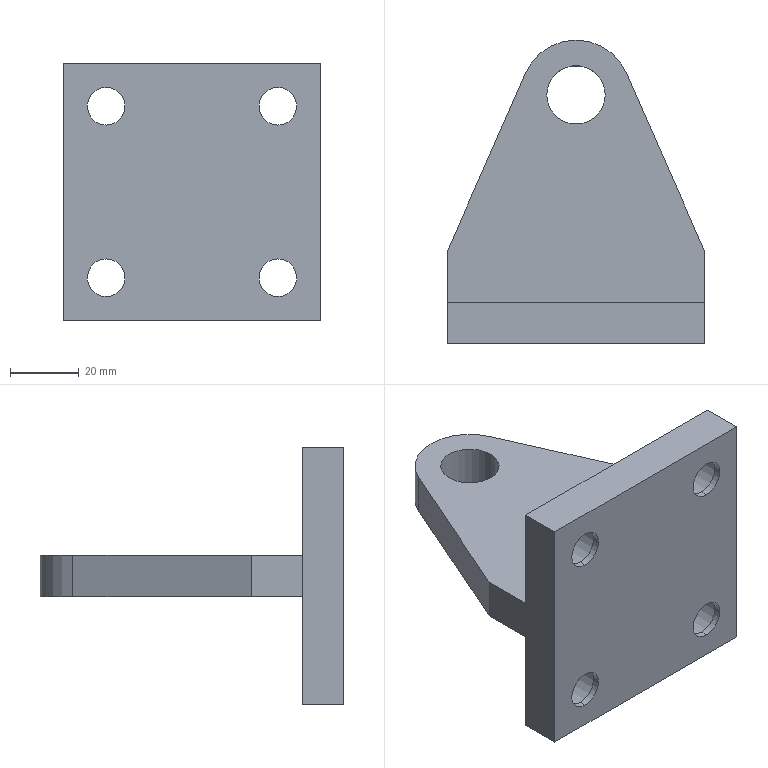Part | SolidWorks | features ICE 3, Extrusion 1, HoleWzd 1 | 2 solids | 36 faces | box 75 x 88.5 x 75 mm | volume 103360 mm3 | cylinder 19 | plane 17 | commonest cylinder face diameters 17 x10 11 x8 32 x1
STEP:
#1=CARTESIAN_POINT('',(-8.5,72.5,-6.));
#2=VERTEX_POINT('',#1);
#3=CARTESIAN_POINT('',(8.5,72.5,-6.));
#4=VERTEX_POINT('',#3);
#5=CARTESIAN_POINT('',(0.,72.5,-6.));
#6=DIRECTION('',(0.,0.,1.));
#7=DIRECTION('',(1.,0.,0.));
#8=AXIS2_PLACEMENT_3D('',#5,#6,#7);
#9=CIRCLE('',#8,8.5);
#10=EDGE_CURVE('',#2,#4,#9,.T.);
#11=ORIENTED_EDGE('',*,*,#10,.F.);
#12=CARTESIAN_POINT('',(-8.5,72.5,6.));
#13=VERTEX_POINT('',#12);
#14=CARTESIAN_POINT('',(-8.5,72.5,-37.5));
#15=DIRECTION('',(0.,0.,1.));
#16=VECTOR('',#15,1000.);
#17=LINE('',#14,#16);
#18=EDGE_CURVE('',#2,#13,#17,.T.);
#19=ORIENTED_EDGE('',*,*,#18,.T.);
#20=CARTESIAN_POINT('',(8.5,72.5,6.));
#21=VERTEX_POINT('',#20);
#22=CARTESIAN_POINT('',(0.,72.5,6.));
#23=DIRECTION('',(0.,0.,1.));
#24=DIRECTION('',(1.,0.,0.));
#25=AXIS2_PLACEMENT_3D('',#22,#23,#24);
#26=CIRCLE('',#25,8.5);
#27=EDGE_CURVE('',#13,#21,#26,.T.);
#28=ORIENTED_EDGE('',*,*,#27,.T.);
#29=CARTESIAN_POINT('',(8.5,72.5,-37.5));
#30=DIRECTION('',(0.,0.,1.));
#31=VECTOR('',#30,1000.);
#32=LINE('',#29,#31);
#33=EDGE_CURVE('',#4,#21,#32,.T.);
#34=ORIENTED_EDGE('',*,*,#33,.F.);
#35=EDGE_LOOP('',(#11,#19,#28,#34));
#36=FACE_OUTER_BOUND('',#35,.T.);
#37=CARTESIAN_POINT('',(0.,72.5,-37.5));
#38=DIRECTION('',(0.,0.,1.));
#39=DIRECTION('',(1.,0.,0.));
#40=AXIS2_PLACEMENT_3D('',#37,#38,#39);
#41=CYLINDRICAL_SURFACE('',#40,8.5);
#42=ADVANCED_FACE('',(#36),#41,.F.);
#43=CARTESIAN_POINT('',(37.5,27.,-6.));
#44=VERTEX_POINT('',#43);
#45=CARTESIAN_POINT('',(37.5,12.,-6.));
#46=VERTEX_POINT('',#45);
#47=CARTESIAN_POINT('',(37.5,88.5,-6.));
#48=DIRECTION('',(0.,-1.,0.));
#49=VECTOR('',#48,1000.);
#50=LINE('',#47,#49);
#51=EDGE_CURVE('',#44,#46,#50,.T.);
#52=ORIENTED_EDGE('',*,*,#51,.F.);
#53=CARTESIAN_POINT('',(37.5,27.,6.));
#54=VERTEX_POINT('',#53);
#55=CARTESIAN_POINT('',(37.5,27.,-37.5));
#56=DIRECTION('',(0.,0.,1.));
#57=VECTOR('',#56,1000.);
#58=LINE('',#55,#57);
#59=EDGE_CURVE('',#44,#54,#58,.T.);
#60=ORIENTED_EDGE('',*,*,#59,.T.);
#61=CARTESIAN_POINT('',(37.5,12.,6.));
#62=VERTEX_POINT('',#61);
#63=CARTESIAN_POINT('',(37.5,88.5,6.));
#64=DIRECTION('',(0.,-1.,0.));
#65=VECTOR('',#64,1000.);
#66=LINE('',#63,#65);
#67=EDGE_CURVE('',#54,#62,#66,.T.);
#68=ORIENTED_EDGE('',*,*,#67,.T.);
#69=CARTESIAN_POINT('',(37.5,12.,-6.));
#70=DIRECTION('',(0.,0.,-1.));
#71=VECTOR('',#70,1000.);
#72=LINE('',#69,#71);
#73=EDGE_CURVE('',#62,#46,#72,.T.);
#74=ORIENTED_EDGE('',*,*,#73,.T.);
#75=EDGE_LOOP('',(#52,#60,#68,#74));
#76=FACE_OUTER_BOUND('',#75,.T.);
#77=CARTESIAN_POINT('',(37.5,88.5,-6.));
#78=DIRECTION('',(-1.,0.,0.));
#79=DIRECTION('',(0.,0.,1.));
#80=AXIS2_PLACEMENT_3D('',#77,#78,#79);
#81=PLANE('',#80);
#82=ADVANCED_FACE('',(#76),#81,.F.);
#83=CARTESIAN_POINT('',(0.,72.5,-6.));
#84=DIRECTION('',(0.,0.,1.));
#85=DIRECTION('',(1.,0.,0.));
#86=AXIS2_PLACEMENT_3D('',#83,#84,#85);
#87=CIRCLE('',#86,8.5);
#88=EDGE_CURVE('',#4,#2,#87,.T.);
#89=ORIENTED_EDGE('',*,*,#88,.T.);
#90=ORIENTED_EDGE('',*,*,#10,.T.);
#91=EDGE_LOOP('',(#89,#90));
#92=FACE_BOUND('',#91,.T.);
#93=CARTESIAN_POINT('',(-37.5,27.,-6.));
#94=VERTEX_POINT('',#93);
#95=CARTESIAN_POINT('',(-37.5,12.,-6.));
#96=VERTEX_POINT('',#95);
#97=CARTESIAN_POINT('',(-37.5,88.5,-6.));
#98=DIRECTION('',(0.,-1.,0.));
#99=VECTOR('',#98,1000.);
#100=LINE('',#97,#99);
#101=EDGE_CURVE('',#94,#96,#100,.T.);
#102=ORIENTED_EDGE('',*,*,#101,.F.);
#103=CARTESIAN_POINT('',(-14.645,78.944,-6.));
#104=VERTEX_POINT('',#103);
#105=CARTESIAN_POINT('',(-14.829,78.525,-6.));
#106=DIRECTION('',(0.4027,0.9153,0.));
#107=VECTOR('',#106,1000.);
#108=LINE('',#105,#107);
#109=EDGE_CURVE('',#94,#104,#108,.T.);
#110=ORIENTED_EDGE('',*,*,#109,.T.);
#111=CARTESIAN_POINT('',(14.645,78.944,-6.));
#112=VERTEX_POINT('',#111);
#113=CARTESIAN_POINT('',(0.,72.5,-6.));
#114=DIRECTION('',(0.,0.,-1.));
#115=DIRECTION('',(1.,0.,0.));
#116=AXIS2_PLACEMENT_3D('',#113,#114,#115);
#117=CIRCLE('',#116,16.);
#118=EDGE_CURVE('',#104,#112,#117,.T.);
#119=ORIENTED_EDGE('',*,*,#118,.T.);
#120=CARTESIAN_POINT('',(2.665,106.172,-6.));
#121=DIRECTION('',(0.4027,-0.9153,0.));
#122=VECTOR('',#121,1000.);
#123=LINE('',#120,#122);
#124=EDGE_CURVE('',#112,#44,#123,.T.);
#125=ORIENTED_EDGE('',*,*,#124,.T.);
#126=ORIENTED_EDGE('',*,*,#51,.T.);
#127=CARTESIAN_POINT('',(-37.5,12.,-6.));
#128=DIRECTION('',(-1.,0.,0.));
#129=VECTOR('',#128,1000.);
#130=LINE('',#127,#129);
#131=EDGE_CURVE('',#46,#96,#130,.T.);
#132=ORIENTED_EDGE('',*,*,#131,.T.);
#133=EDGE_LOOP('',(#102,#110,#119,#125,#126,#132));
#134=FACE_OUTER_BOUND('',#133,.T.);
#135=CARTESIAN_POINT('',(-37.5,88.5,-6.));
#136=DIRECTION('',(0.,0.,1.));
#137=DIRECTION('',(1.,0.,0.));
#138=AXIS2_PLACEMENT_3D('',#135,#136,#137);
#139=PLANE('',#138);
#140=ADVANCED_FACE('',(#92,#134),#139,.F.);
#141=CARTESIAN_POINT('',(-37.5,27.,6.));
#142=VERTEX_POINT('',#141);
#143=CARTESIAN_POINT('',(-37.5,12.,6.));
#144=VERTEX_POINT('',#143);
#145=CARTESIAN_POINT('',(-37.5,88.5,6.));
#146=DIRECTION('',(0.,-1.,0.));
#147=VECTOR('',#146,1000.);
#148=LINE('',#145,#147);
#149=EDGE_CURVE('',#142,#144,#148,.T.);
#150=ORIENTED_EDGE('',*,*,#149,.F.);
#151=CARTESIAN_POINT('',(-37.5,27.,-37.5));
#152=DIRECTION('',(0.,0.,1.));
#153=VECTOR('',#152,1000.);
#154=LINE('',#151,#153);
#155=EDGE_CURVE('',#94,#142,#154,.T.);
#156=ORIENTED_EDGE('',*,*,#155,.F.);
#157=ORIENTED_EDGE('',*,*,#101,.T.);
#158=CARTESIAN_POINT('',(-37.5,12.,-6.));
#159=DIRECTION('',(0.,0.,1.));
#160=VECTOR('',#159,1000.);
#161=LINE('',#158,#160);
#162=EDGE_CURVE('',#96,#144,#161,.T.);
#163=ORIENTED_EDGE('',*,*,#162,.T.);
#164=EDGE_LOOP('',(#150,#156,#157,#163));
#165=FACE_OUTER_BOUND('',#164,.T.);
#166=CARTESIAN_POINT('',(-37.5,88.5,-6.));
#167=DIRECTION('',(1.,0.,0.));
#168=DIRECTION('',(0.,0.,-1.));
#169=AXIS2_PLACEMENT_3D('',#166,#167,#168);
#170=PLANE('',#169);
#171=ADVANCED_FACE('',(#165),#170,.F.);
#172=CARTESIAN_POINT('',(0.,72.5,6.));
#173=DIRECTION('',(0.,0.,1.));
#174=DIRECTION('',(1.,0.,0.));
#175=AXIS2_PLACEMENT_3D('',#172,#173,#174);
#176=CIRCLE('',#175,8.5);
#177=EDGE_CURVE('',#21,#13,#176,.T.);
#178=ORIENTED_EDGE('',*,*,#177,.F.);
#179=ORIENTED_EDGE('',*,*,#27,.F.);
#180=EDGE_LOOP('',(#178,#179));
#181=FACE_BOUND('',#180,.T.);
#182=CARTESIAN_POINT('',(-14.645,78.944,6.));
#183=VERTEX_POINT('',#182);
#184=CARTESIAN_POINT('',(14.645,78.944,6.));
#185=VERTEX_POINT('',#184);
#186=CARTESIAN_POINT('',(0.,72.5,6.));
#187=DIRECTION('',(0.,0.,-1.));
#188=DIRECTION('',(1.,0.,0.));
#189=AXIS2_PLACEMENT_3D('',#186,#187,#188);
#190=CIRCLE('',#189,16.);
#191=EDGE_CURVE('',#183,#185,#190,.T.);
#192=ORIENTED_EDGE('',*,*,#191,.F.);
#193=CARTESIAN_POINT('',(-37.5,27.,6.));
#194=DIRECTION('',(0.4027,0.9153,0.));
#195=VECTOR('',#194,1000.);
#196=LINE('',#193,#195);
#197=EDGE_CURVE('',#142,#183,#196,.T.);
#198=ORIENTED_EDGE('',*,*,#197,.F.);
#199=ORIENTED_EDGE('',*,*,#149,.T.);
#200=CARTESIAN_POINT('',(-37.5,12.,6.));
#201=DIRECTION('',(1.,0.,0.));
#202=VECTOR('',#201,1000.);
#203=LINE('',#200,#202);
#204=EDGE_CURVE('',#144,#62,#203,.T.);
#205=ORIENTED_EDGE('',*,*,#204,.T.);
#206=ORIENTED_EDGE('',*,*,#67,.F.);
#207=CARTESIAN_POINT('',(37.5,27.,6.));
#208=DIRECTION('',(0.4027,-0.9153,0.));
#209=VECTOR('',#208,1000.);
#210=LINE('',#207,#209);
#211=EDGE_CURVE('',#185,#54,#210,.T.);
#212=ORIENTED_EDGE('',*,*,#211,.F.);
#213=EDGE_LOOP('',(#192,#198,#199,#205,#206,#212));
#214=FACE_OUTER_BOUND('',#213,.T.);
#215=CARTESIAN_POINT('',(-37.5,88.5,6.));
#216=DIRECTION('',(0.,0.,-1.));
#217=DIRECTION('',(-1.,0.,0.));
#218=AXIS2_PLACEMENT_3D('',#215,#216,#217);
#219=PLANE('',#218);
#220=ADVANCED_FACE('',(#181,#214),#219,.F.);
#221=ORIENTED_EDGE('',*,*,#73,.F.);
#222=ORIENTED_EDGE('',*,*,#204,.F.);
#223=ORIENTED_EDGE('',*,*,#162,.F.);
#224=ORIENTED_EDGE('',*,*,#131,.F.);
#225=EDGE_LOOP('',(#221,#222,#223,#224));
#226=FACE_OUTER_BOUND('',#225,.T.);
#227=CARTESIAN_POINT('',(0.,12.,0.));
#228=DIRECTION('',(0.,1.,0.));
#229=DIRECTION('',(0.,0.,1.));
#230=AXIS2_PLACEMENT_3D('',#227,#228,#229);
#231=PLANE('',#230);
#232=ADVANCED_FACE('',(#226),#231,.F.);
#233=ORIENTED_EDGE('',*,*,#18,.F.);
#234=ORIENTED_EDGE('',*,*,#88,.F.);
#235=ORIENTED_EDGE('',*,*,#33,.T.);
#236=ORIENTED_EDGE('',*,*,#177,.T.);
#237=EDGE_LOOP('',(#233,#234,#235,#236));
#238=FACE_OUTER_BOUND('',#237,.T.);
#239=CARTESIAN_POINT('',(0.,72.5,-37.5));
#240=DIRECTION('',(0.,0.,1.));
#241=DIRECTION('',(1.,0.,0.));
#242=AXIS2_PLACEMENT_3D('',#239,#240,#241);
#243=CYLINDRICAL_SURFACE('',#242,8.5);
#244=ADVANCED_FACE('',(#238),#243,.F.);
#245=ORIENTED_EDGE('',*,*,#155,.T.);
#246=ORIENTED_EDGE('',*,*,#197,.T.);
#247=CARTESIAN_POINT('',(-14.645,78.944,-37.5));
#248=DIRECTION('',(0.,0.,1.));
#249=VECTOR('',#248,1000.);
#250=LINE('',#247,#249);
#251=EDGE_CURVE('',#104,#183,#250,.T.);
#252=ORIENTED_EDGE('',*,*,#251,.F.);
#253=ORIENTED_EDGE('',*,*,#109,.F.);
#254=EDGE_LOOP('',(#245,#246,#252,#253));
#255=FACE_OUTER_BOUND('',#254,.T.);
#256=CARTESIAN_POINT('',(-37.5,27.,-37.5));
#257=DIRECTION('',(0.9153,-0.4027,0.));
#258=DIRECTION('',(0.4027,0.9153,0.));
#259=AXIS2_PLACEMENT_3D('',#256,#257,#258);
#260=PLANE('',#259);
#261=ADVANCED_FACE('',(#255),#260,.F.);
#262=CARTESIAN_POINT('',(14.645,78.944,-37.5));
#263=DIRECTION('',(0.,0.,1.));
#264=VECTOR('',#263,1000.);
#265=LINE('',#262,#264);
#266=EDGE_CURVE('',#112,#185,#265,.T.);
#267=ORIENTED_EDGE('',*,*,#266,.T.);
#268=ORIENTED_EDGE('',*,*,#211,.T.);
#269=ORIENTED_EDGE('',*,*,#59,.F.);
#270=ORIENTED_EDGE('',*,*,#124,.F.);
#271=EDGE_LOOP('',(#267,#268,#269,#270));
#272=FACE_OUTER_BOUND('',#271,.T.);
#273=CARTESIAN_POINT('',(37.5,27.,-37.5));
#274=DIRECTION('',(-0.9153,-0.4027,0.));
#275=DIRECTION('',(0.4027,-0.9153,0.));
#276=AXIS2_PLACEMENT_3D('',#273,#274,#275);
#277=PLANE('',#276);
#278=ADVANCED_FACE('',(#272),#277,.F.);
#279=ORIENTED_EDGE('',*,*,#251,.T.);
#280=ORIENTED_EDGE('',*,*,#191,.T.);
#281=ORIENTED_EDGE('',*,*,#266,.F.);
#282=ORIENTED_EDGE('',*,*,#118,.F.);
#283=EDGE_LOOP('',(#279,#280,#281,#282));
#284=FACE_OUTER_BOUND('',#283,.T.);
#285=CARTESIAN_POINT('',(0.,72.5,-37.5));
#286=DIRECTION('',(0.,0.,1.));
#287=DIRECTION('',(1.,0.,0.));
#288=AXIS2_PLACEMENT_3D('',#285,#286,#287);
#289=CYLINDRICAL_SURFACE('',#288,16.);
#290=ADVANCED_FACE('',(#284),#289,.T.);
#291=CLOSED_SHELL('',(#42,#82,#140,#171,#220,#232,#244,#261,#278,#290));
#292=MANIFOLD_SOLID_BREP('',#291);
#293=CARTESIAN_POINT('',(25.,2.,16.5));
#294=VERTEX_POINT('',#293);
#295=CARTESIAN_POINT('',(25.,2.,33.5));
#296=VERTEX_POINT('',#295);
#297=CARTESIAN_POINT('',(25.,2.,25.));
#298=DIRECTION('',(0.,1.,0.));
#299=DIRECTION('',(0.,0.,1.));
#300=AXIS2_PLACEMENT_3D('',#297,#298,#299);
#301=CIRCLE('',#300,8.5);
#302=EDGE_CURVE('',#294,#296,#301,.T.);
#303=ORIENTED_EDGE('',*,*,#302,.F.);
#304=CARTESIAN_POINT('',(25.,12.,16.5));
#305=VERTEX_POINT('',#304);
#306=CARTESIAN_POINT('',(25.,12.,16.5));
#307=DIRECTION('',(0.,1.,0.));
#308=VECTOR('',#307,1000.);
#309=LINE('',#306,#308);
#310=EDGE_CURVE('',#294,#305,#309,.T.);
#311=ORIENTED_EDGE('',*,*,#310,.T.);
#312=CARTESIAN_POINT('',(25.,12.,33.5));
#313=VERTEX_POINT('',#312);
#314=CARTESIAN_POINT('',(25.,12.,25.));
#315=DIRECTION('',(0.,1.,0.));
#316=DIRECTION('',(0.,0.,1.));
#317=AXIS2_PLACEMENT_3D('',#314,#315,#316);
#318=CIRCLE('',#317,8.5);
#319=EDGE_CURVE('',#305,#313,#318,.T.);
#320=ORIENTED_EDGE('',*,*,#319,.T.);
#321=CARTESIAN_POINT('',(25.,12.,33.5));
#322=DIRECTION('',(0.,1.,0.));
#323=VECTOR('',#322,1000.);
#324=LINE('',#321,#323);
#325=EDGE_CURVE('',#296,#313,#324,.T.);
#326=ORIENTED_EDGE('',*,*,#325,.F.);
#327=EDGE_LOOP('',(#303,#311,#320,#326));
#328=FACE_OUTER_BOUND('',#327,.T.);
#329=CARTESIAN_POINT('',(25.,12.,25.));
#330=DIRECTION('',(0.,1.,0.));
#331=DIRECTION('',(0.,0.,1.));
#332=AXIS2_PLACEMENT_3D('',#329,#330,#331);
#333=CYLINDRICAL_SURFACE('',#332,8.5);
#334=ADVANCED_FACE('',(#328),#333,.F.);
#335=CARTESIAN_POINT('',(25.,0.,19.5));
#336=VERTEX_POINT('',#335);
#337=CARTESIAN_POINT('',(25.,0.,30.5));
#338=VERTEX_POINT('',#337);
#339=CARTESIAN_POINT('',(25.,0.,25.));
#340=DIRECTION('',(0.,1.,0.));
#341=DIRECTION('',(0.,0.,1.));
#342=AXIS2_PLACEMENT_3D('',#339,#340,#341);
#343=CIRCLE('',#342,5.5);
#344=EDGE_CURVE('',#336,#338,#343,.T.);
#345=ORIENTED_EDGE('',*,*,#344,.F.);
#346=CARTESIAN_POINT('',(25.,2.,19.5));
#347=VERTEX_POINT('',#346);
#348=CARTESIAN_POINT('',(25.,12.,19.5));
#349=DIRECTION('',(0.,1.,0.));
#350=VECTOR('',#349,1000.);
#351=LINE('',#348,#350);
#352=EDGE_CURVE('',#336,#347,#351,.T.);
#353=ORIENTED_EDGE('',*,*,#352,.T.);
#354=CARTESIAN_POINT('',(25.,2.,30.5));
#355=VERTEX_POINT('',#354);
#356=CARTESIAN_POINT('',(25.,2.,25.));
#357=DIRECTION('',(0.,1.,0.));
#358=DIRECTION('',(0.,0.,1.));
#359=AXIS2_PLACEMENT_3D('',#356,#357,#358);
#360=CIRCLE('',#359,5.5);
#361=EDGE_CURVE('',#347,#355,#360,.T.);
#362=ORIENTED_EDGE('',*,*,#361,.T.);
#363=CARTESIAN_POINT('',(25.,12.,30.5));
#364=DIRECTION('',(0.,1.,0.));
#365=VECTOR('',#364,1000.);
#366=LINE('',#363,#365);
#367=EDGE_CURVE('',#338,#355,#366,.T.);
#368=ORIENTED_EDGE('',*,*,#367,.F.);
#369=EDGE_LOOP('',(#345,#353,#362,#368));
#370=FACE_OUTER_BOUND('',#369,.T.);
#371=CARTESIAN_POINT('',(25.,12.,25.));
#372=DIRECTION('',(0.,1.,0.));
#373=DIRECTION('',(0.,0.,1.));
#374=AXIS2_PLACEMENT_3D('',#371,#372,#373);
#375=CYLINDRICAL_SURFACE('',#374,5.5);
#376=ADVANCED_FACE('',(#370),#375,.F.);
#377=CARTESIAN_POINT('',(-25.,2.,-33.5));
#378=VERTEX_POINT('',#377);
#379=CARTESIAN_POINT('',(-25.,2.,-16.5));
#380=VERTEX_POINT('',#379);
#381=CARTESIAN_POINT('',(-25.,2.,-25.));
#382=DIRECTION('',(0.,1.,0.));
#383=DIRECTION('',(0.,0.,1.));
#384=AXIS2_PLACEMENT_3D('',#381,#382,#383);
#385=CIRCLE('',#384,8.5);
#386=EDGE_CURVE('',#378,#380,#385,.T.);
#387=ORIENTED_EDGE('',*,*,#386,.F.);
#388=CARTESIAN_POINT('',(-25.,12.,-33.5));
#389=VERTEX_POINT('',#388);
#390=CARTESIAN_POINT('',(-25.,12.,-33.5));
#391=DIRECTION('',(0.,1.,0.));
#392=VECTOR('',#391,1000.);
#393=LINE('',#390,#392);
#394=EDGE_CURVE('',#378,#389,#393,.T.);
#395=ORIENTED_EDGE('',*,*,#394,.T.);
#396=CARTESIAN_POINT('',(-25.,12.,-16.5));
#397=VERTEX_POINT('',#396);
#398=CARTESIAN_POINT('',(-25.,12.,-25.));
#399=DIRECTION('',(0.,1.,0.));
#400=DIRECTION('',(0.,0.,1.));
#401=AXIS2_PLACEMENT_3D('',#398,#399,#400);
#402=CIRCLE('',#401,8.5);
#403=EDGE_CURVE('',#389,#397,#402,.T.);
#404=ORIENTED_EDGE('',*,*,#403,.T.);
#405=CARTESIAN_POINT('',(-25.,12.,-16.5));
#406=DIRECTION('',(0.,1.,0.));
#407=VECTOR('',#406,1000.);
#408=LINE('',#405,#407);
#409=EDGE_CURVE('',#380,#397,#408,.T.);
#410=ORIENTED_EDGE('',*,*,#409,.F.);
#411=EDGE_LOOP('',(#387,#395,#404,#410));
#412=FACE_OUTER_BOUND('',#411,.T.);
#413=CARTESIAN_POINT('',(-25.,12.,-25.));
#414=DIRECTION('',(0.,1.,0.));
#415=DIRECTION('',(0.,0.,1.));
#416=AXIS2_PLACEMENT_3D('',#413,#414,#415);
#417=CYLINDRICAL_SURFACE('',#416,8.5);
#418=ADVANCED_FACE('',(#412),#417,.F.);
#419=CARTESIAN_POINT('',(-25.,0.,-30.5));
#420=VERTEX_POINT('',#419);
#421=CARTESIAN_POINT('',(-25.,0.,-19.5));
#422=VERTEX_POINT('',#421);
#423=CARTESIAN_POINT('',(-25.,0.,-25.));
#424=DIRECTION('',(0.,1.,0.));
#425=DIRECTION('',(0.,0.,1.));
#426=AXIS2_PLACEMENT_3D('',#423,#424,#425);
#427=CIRCLE('',#426,5.5);
#428=EDGE_CURVE('',#420,#422,#427,.T.);
#429=ORIENTED_EDGE('',*,*,#428,.F.);
#430=CARTESIAN_POINT('',(-25.,2.,-30.5));
#431=VERTEX_POINT('',#430);
#432=CARTESIAN_POINT('',(-25.,12.,-30.5));
#433=DIRECTION('',(0.,1.,0.));
#434=VECTOR('',#433,1000.);
#435=LINE('',#432,#434);
#436=EDGE_CURVE('',#420,#431,#435,.T.);
#437=ORIENTED_EDGE('',*,*,#436,.T.);
#438=CARTESIAN_POINT('',(-25.,2.,-19.5));
#439=VERTEX_POINT('',#438);
#440=CARTESIAN_POINT('',(-25.,2.,-25.));
#441=DIRECTION('',(0.,1.,0.));
#442=DIRECTION('',(0.,0.,1.));
#443=AXIS2_PLACEMENT_3D('',#440,#441,#442);
#444=CIRCLE('',#443,5.5);
#445=EDGE_CURVE('',#431,#439,#444,.T.);
#446=ORIENTED_EDGE('',*,*,#445,.T.);
#447=CARTESIAN_POINT('',(-25.,12.,-19.5));
#448=DIRECTION('',(0.,1.,0.));
#449=VECTOR('',#448,1000.);
#450=LINE('',#447,#449);
#451=EDGE_CURVE('',#422,#439,#450,.T.);
#452=ORIENTED_EDGE('',*,*,#451,.F.);
#453=EDGE_LOOP('',(#429,#437,#446,#452));
#454=FACE_OUTER_BOUND('',#453,.T.);
#455=CARTESIAN_POINT('',(-25.,12.,-25.));
#456=DIRECTION('',(0.,1.,0.));
#457=DIRECTION('',(0.,0.,1.));
#458=AXIS2_PLACEMENT_3D('',#455,#456,#457);
#459=CYLINDRICAL_SURFACE('',#458,5.5);
#460=ADVANCED_FACE('',(#454),#459,.F.);
#461=CARTESIAN_POINT('',(-25.,2.,16.5));
#462=VERTEX_POINT('',#461);
#463=CARTESIAN_POINT('',(-25.,2.,33.5));
#464=VERTEX_POINT('',#463);
#465=CARTESIAN_POINT('',(-25.,2.,25.));
#466=DIRECTION('',(0.,1.,0.));
#467=DIRECTION('',(0.,0.,1.));
#468=AXIS2_PLACEMENT_3D('',#465,#466,#467);
#469=CIRCLE('',#468,8.5);
#470=EDGE_CURVE('',#462,#464,#469,.T.);
#471=ORIENTED_EDGE('',*,*,#470,.F.);
#472=CARTESIAN_POINT('',(-25.,12.,16.5));
#473=VERTEX_POINT('',#472);
#474=CARTESIAN_POINT('',(-25.,12.,16.5));
#475=DIRECTION('',(0.,1.,0.));
#476=VECTOR('',#475,1000.);
#477=LINE('',#474,#476);
#478=EDGE_CURVE('',#462,#473,#477,.T.);
#479=ORIENTED_EDGE('',*,*,#478,.T.);
#480=CARTESIAN_POINT('',(-25.,12.,33.5));
#481=VERTEX_POINT('',#480);
#482=CARTESIAN_POINT('',(-25.,12.,25.));
#483=DIRECTION('',(0.,1.,0.));
#484=DIRECTION('',(0.,0.,1.));
#485=AXIS2_PLACEMENT_3D('',#482,#483,#484);
#486=CIRCLE('',#485,8.5);
#487=EDGE_CURVE('',#473,#481,#486,.T.);
#488=ORIENTED_EDGE('',*,*,#487,.T.);
#489=CARTESIAN_POINT('',(-25.,12.,33.5));
#490=DIRECTION('',(0.,1.,0.));
#491=VECTOR('',#490,1000.);
#492=LINE('',#489,#491);
#493=EDGE_CURVE('',#464,#481,#492,.T.);
#494=ORIENTED_EDGE('',*,*,#493,.F.);
#495=EDGE_LOOP('',(#471,#479,#488,#494));
#496=FACE_OUTER_BOUND('',#495,.T.);
#497=CARTESIAN_POINT('',(-25.,12.,25.));
#498=DIRECTION('',(0.,1.,0.));
#499=DIRECTION('',(0.,0.,1.));
#500=AXIS2_PLACEMENT_3D('',#497,#498,#499);
#501=CYLINDRICAL_SURFACE('',#500,8.5);
#502=ADVANCED_FACE('',(#496),#501,.F.);
#503=CARTESIAN_POINT('',(-25.,0.,19.5));
#504=VERTEX_POINT('',#503);
#505=CARTESIAN_POINT('',(-25.,0.,30.5));
#506=VERTEX_POINT('',#505);
#507=CARTESIAN_POINT('',(-25.,0.,25.));
#508=DIRECTION('',(0.,1.,0.));
#509=DIRECTION('',(0.,0.,1.));
#510=AXIS2_PLACEMENT_3D('',#507,#508,#509);
#511=CIRCLE('',#510,5.5);
#512=EDGE_CURVE('',#504,#506,#511,.T.);
#513=ORIENTED_EDGE('',*,*,#512,.F.);
#514=CARTESIAN_POINT('',(-25.,2.,19.5));
#515=VERTEX_POINT('',#514);
#516=CARTESIAN_POINT('',(-25.,12.,19.5));
#517=DIRECTION('',(0.,1.,0.));
#518=VECTOR('',#517,1000.);
#519=LINE('',#516,#518);
#520=EDGE_CURVE('',#504,#515,#519,.T.);
#521=ORIENTED_EDGE('',*,*,#520,.T.);
#522=CARTESIAN_POINT('',(-25.,2.,30.5));
#523=VERTEX_POINT('',#522);
#524=CARTESIAN_POINT('',(-25.,2.,25.));
#525=DIRECTION('',(0.,1.,0.));
#526=DIRECTION('',(0.,0.,1.));
#527=AXIS2_PLACEMENT_3D('',#524,#525,#526);
#528=CIRCLE('',#527,5.5);
#529=EDGE_CURVE('',#515,#523,#528,.T.);
#530=ORIENTED_EDGE('',*,*,#529,.T.);
#531=CARTESIAN_POINT('',(-25.,12.,30.5));
#532=DIRECTION('',(0.,1.,0.));
#533=VECTOR('',#532,1000.);
#534=LINE('',#531,#533);
#535=EDGE_CURVE('',#506,#523,#534,.T.);
#536=ORIENTED_EDGE('',*,*,#535,.F.);
#537=EDGE_LOOP('',(#513,#521,#530,#536));
#538=FACE_OUTER_BOUND('',#537,.T.);
#539=CARTESIAN_POINT('',(-25.,12.,25.));
#540=DIRECTION('',(0.,1.,0.));
#541=DIRECTION('',(0.,0.,1.));
#542=AXIS2_PLACEMENT_3D('',#539,#540,#541);
#543=CYLINDRICAL_SURFACE('',#542,5.5);
#544=ADVANCED_FACE('',(#538),#543,.F.);
#545=CARTESIAN_POINT('',(25.,2.,-33.5));
#546=VERTEX_POINT('',#545);
#547=CARTESIAN_POINT('',(25.,2.,-16.5));
#548=VERTEX_POINT('',#547);
#549=CARTESIAN_POINT('',(25.,2.,-25.));
#550=DIRECTION('',(0.,1.,0.));
#551=DIRECTION('',(0.,0.,1.));
#552=AXIS2_PLACEMENT_3D('',#549,#550,#551);
#553=CIRCLE('',#552,8.5);
#554=EDGE_CURVE('',#546,#548,#553,.T.);
#555=ORIENTED_EDGE('',*,*,#554,.F.);
#556=CARTESIAN_POINT('',(25.,12.,-33.5));
#557=VERTEX_POINT('',#556);
#558=CARTESIAN_POINT('',(25.,12.,-33.5));
#559=DIRECTION('',(0.,1.,0.));
#560=VECTOR('',#559,1000.);
#561=LINE('',#558,#560);
#562=EDGE_CURVE('',#546,#557,#561,.T.);
#563=ORIENTED_EDGE('',*,*,#562,.T.);
#564=CARTESIAN_POINT('',(25.,12.,-16.5));
#565=VERTEX_POINT('',#564);
#566=CARTESIAN_POINT('',(25.,12.,-25.));
#567=DIRECTION('',(0.,1.,0.));
#568=DIRECTION('',(0.,0.,1.));
#569=AXIS2_PLACEMENT_3D('',#566,#567,#568);
#570=CIRCLE('',#569,8.5);
#571=EDGE_CURVE('',#557,#565,#570,.T.);
#572=ORIENTED_EDGE('',*,*,#571,.T.);
#573=CARTESIAN_POINT('',(25.,12.,-16.5));
#574=DIRECTION('',(0.,1.,0.));
#575=VECTOR('',#574,1000.);
#576=LINE('',#573,#575);
#577=EDGE_CURVE('',#548,#565,#576,.T.);
#578=ORIENTED_EDGE('',*,*,#577,.F.);
#579=EDGE_LOOP('',(#555,#563,#572,#578));
#580=FACE_OUTER_BOUND('',#579,.T.);
#581=CARTESIAN_POINT('',(25.,12.,-25.));
#582=DIRECTION('',(0.,1.,0.));
#583=DIRECTION('',(0.,0.,1.));
#584=AXIS2_PLACEMENT_3D('',#581,#582,#583);
#585=CYLINDRICAL_SURFACE('',#584,8.5);
#586=ADVANCED_FACE('',(#580),#585,.F.);
#587=CARTESIAN_POINT('',(25.,0.,-30.5));
#588=VERTEX_POINT('',#587);
#589=CARTESIAN_POINT('',(25.,0.,-19.5));
#590=VERTEX_POINT('',#589);
#591=CARTESIAN_POINT('',(25.,0.,-25.));
#592=DIRECTION('',(0.,1.,0.));
#593=DIRECTION('',(0.,0.,1.));
#594=AXIS2_PLACEMENT_3D('',#591,#592,#593);
#595=CIRCLE('',#594,5.5);
#596=EDGE_CURVE('',#588,#590,#595,.T.);
#597=ORIENTED_EDGE('',*,*,#596,.F.);
#598=CARTESIAN_POINT('',(25.,2.,-30.5));
#599=VERTEX_POINT('',#598);
#600=CARTESIAN_POINT('',(25.,12.,-30.5));
#601=DIRECTION('',(0.,1.,0.));
#602=VECTOR('',#601,1000.);
#603=LINE('',#600,#602);
#604=EDGE_CURVE('',#588,#599,#603,.T.);
#605=ORIENTED_EDGE('',*,*,#604,.T.);
#606=CARTESIAN_POINT('',(25.,2.,-19.5));
#607=VERTEX_POINT('',#606);
#608=CARTESIAN_POINT('',(25.,2.,-25.));
#609=DIRECTION('',(0.,1.,0.));
#610=DIRECTION('',(0.,0.,1.));
#611=AXIS2_PLACEMENT_3D('',#608,#609,#610);
#612=CIRCLE('',#611,5.5);
#613=EDGE_CURVE('',#599,#607,#612,.T.);
#614=ORIENTED_EDGE('',*,*,#613,.T.);
#615=CARTESIAN_POINT('',(25.,12.,-19.5));
#616=DIRECTION('',(0.,1.,0.));
#617=VECTOR('',#616,1000.);
#618=LINE('',#615,#617);
#619=EDGE_CURVE('',#590,#607,#618,.T.);
#620=ORIENTED_EDGE('',*,*,#619,.F.);
#621=EDGE_LOOP('',(#597,#605,#614,#620));
#622=FACE_OUTER_BOUND('',#621,.T.);
#623=CARTESIAN_POINT('',(25.,12.,-25.));
#624=DIRECTION('',(0.,1.,0.));
#625=DIRECTION('',(0.,0.,1.));
#626=AXIS2_PLACEMENT_3D('',#623,#624,#625);
#627=CYLINDRICAL_SURFACE('',#626,5.5);
#628=ADVANCED_FACE('',(#622),#627,.F.);
#629=CARTESIAN_POINT('',(37.5,0.,37.5));
#630=VERTEX_POINT('',#629);
#631=CARTESIAN_POINT('',(37.5,0.,-37.5));
#632=VERTEX_POINT('',#631);
#633=CARTESIAN_POINT('',(37.5,0.,-37.5));
#634=DIRECTION('',(0.,0.,-1.));
#635=VECTOR('',#634,1000.);
#636=LINE('',#633,#635);
#637=EDGE_CURVE('',#630,#632,#636,.T.);
#638=ORIENTED_EDGE('',*,*,#637,.T.);
#639=CARTESIAN_POINT('',(37.5,12.,-37.5));
#640=VERTEX_POINT('',#639);
#641=CARTESIAN_POINT('',(37.5,12.,-37.5));
#642=DIRECTION('',(0.,-1.,0.));
#643=VECTOR('',#642,1000.);
#644=LINE('',#641,#643);
#645=EDGE_CURVE('',#640,#632,#644,.T.);
#646=ORIENTED_EDGE('',*,*,#645,.F.);
#647=CARTESIAN_POINT('',(37.5,12.,37.5));
#648=VERTEX_POINT('',#647);
#649=CARTESIAN_POINT('',(37.5,12.,-37.5));
#650=DIRECTION('',(0.,0.,-1.));
#651=VECTOR('',#650,1000.);
#652=LINE('',#649,#651);
#653=EDGE_CURVE('',#648,#640,#652,.T.);
#654=ORIENTED_EDGE('',*,*,#653,.F.);
#655=CARTESIAN_POINT('',(37.5,12.,37.5));
#656=DIRECTION('',(0.,-1.,0.));
#657=VECTOR('',#656,1000.);
#658=LINE('',#655,#657);
#659=EDGE_CURVE('',#648,#630,#658,.T.);
#660=ORIENTED_EDGE('',*,*,#659,.T.);
#661=EDGE_LOOP('',(#638,#646,#654,#660));
#662=FACE_OUTER_BOUND('',#661,.T.);
#663=CARTESIAN_POINT('',(37.5,12.,-37.5));
#664=DIRECTION('',(-1.,0.,0.));
#665=DIRECTION('',(0.,0.,1.));
#666=AXIS2_PLACEMENT_3D('',#663,#664,#665);
#667=PLANE('',#666);
#668=ADVANCED_FACE('',(#662),#667,.F.);
#669=CARTESIAN_POINT('',(-37.5,0.,-37.5));
#670=VERTEX_POINT('',#669);
#671=CARTESIAN_POINT('',(-37.5,0.,-37.5));
#672=DIRECTION('',(-1.,0.,0.));
#673=VECTOR('',#672,1000.);
#674=LINE('',#671,#673);
#675=EDGE_CURVE('',#632,#670,#674,.T.);
#676=ORIENTED_EDGE('',*,*,#675,.T.);
#677=CARTESIAN_POINT('',(-37.5,12.,-37.5));
#678=VERTEX_POINT('',#677);
#679=CARTESIAN_POINT('',(-37.5,12.,-37.5));
#680=DIRECTION('',(0.,-1.,0.));
#681=VECTOR('',#680,1000.);
#682=LINE('',#679,#681);
#683=EDGE_CURVE('',#678,#670,#682,.T.);
#684=ORIENTED_EDGE('',*,*,#683,.F.);
#685=CARTESIAN_POINT('',(-37.5,12.,-37.5));
#686=DIRECTION('',(-1.,0.,0.));
#687=VECTOR('',#686,1000.);
#688=LINE('',#685,#687);
#689=EDGE_CURVE('',#640,#678,#688,.T.);
#690=ORIENTED_EDGE('',*,*,#689,.F.);
#691=ORIENTED_EDGE('',*,*,#645,.T.);
#692=EDGE_LOOP('',(#676,#684,#690,#691));
#693=FACE_OUTER_BOUND('',#692,.T.);
#694=CARTESIAN_POINT('',(-37.5,12.,-37.5));
#695=DIRECTION('',(0.,0.,1.));
#696=DIRECTION('',(1.,0.,0.));
#697=AXIS2_PLACEMENT_3D('',#694,#695,#696);
#698=PLANE('',#697);
#699=ADVANCED_FACE('',(#693),#698,.F.);
#700=CARTESIAN_POINT('',(-37.5,0.,37.5));
#701=VERTEX_POINT('',#700);
#702=CARTESIAN_POINT('',(-37.5,0.,-37.5));
#703=DIRECTION('',(0.,0.,1.));
#704=VECTOR('',#703,1000.);
#705=LINE('',#702,#704);
#706=EDGE_CURVE('',#670,#701,#705,.T.);
#707=ORIENTED_EDGE('',*,*,#706,.T.);
#708=CARTESIAN_POINT('',(-37.5,12.,37.5));
#709=VERTEX_POINT('',#708);
#710=CARTESIAN_POINT('',(-37.5,12.,37.5));
#711=DIRECTION('',(0.,-1.,0.));
#712=VECTOR('',#711,1000.);
#713=LINE('',#710,#712);
#714=EDGE_CURVE('',#709,#701,#713,.T.);
#715=ORIENTED_EDGE('',*,*,#714,.F.);
#716=CARTESIAN_POINT('',(-37.5,12.,-37.5));
#717=DIRECTION('',(0.,0.,1.));
#718=VECTOR('',#717,1000.);
#719=LINE('',#716,#718);
#720=EDGE_CURVE('',#678,#709,#719,.T.);
#721=ORIENTED_EDGE('',*,*,#720,.F.);
#722=ORIENTED_EDGE('',*,*,#683,.T.);
#723=EDGE_LOOP('',(#707,#715,#721,#722));
#724=FACE_OUTER_BOUND('',#723,.T.);
#725=CARTESIAN_POINT('',(-37.5,12.,-37.5));
#726=DIRECTION('',(1.,0.,0.));
#727=DIRECTION('',(0.,0.,-1.));
#728=AXIS2_PLACEMENT_3D('',#725,#726,#727);
#729=PLANE('',#728);
#730=ADVANCED_FACE('',(#724),#729,.F.);
#731=CARTESIAN_POINT('',(-37.5,0.,37.5));
#732=DIRECTION('',(1.,0.,0.));
#733=VECTOR('',#732,1000.);
#734=LINE('',#731,#733);
#735=EDGE_CURVE('',#701,#630,#734,.T.);
#736=ORIENTED_EDGE('',*,*,#735,.T.);
#737=ORIENTED_EDGE('',*,*,#659,.F.);
#738=CARTESIAN_POINT('',(-37.5,12.,37.5));
#739=DIRECTION('',(1.,0.,0.));
#740=VECTOR('',#739,1000.);
#741=LINE('',#738,#740);
#742=EDGE_CURVE('',#709,#648,#741,.T.);
#743=ORIENTED_EDGE('',*,*,#742,.F.);
#744=ORIENTED_EDGE('',*,*,#714,.T.);
#745=EDGE_LOOP('',(#736,#737,#743,#744));
#746=FACE_OUTER_BOUND('',#745,.T.);
#747=CARTESIAN_POINT('',(-37.5,12.,37.5));
#748=DIRECTION('',(0.,0.,-1.));
#749=DIRECTION('',(-1.,0.,0.));
#750=AXIS2_PLACEMENT_3D('',#747,#748,#749);
#751=PLANE('',#750);
#752=ADVANCED_FACE('',(#746),#751,.F.);
#753=CARTESIAN_POINT('',(25.,12.,25.));
#754=DIRECTION('',(0.,1.,0.));
#755=DIRECTION('',(0.,0.,1.));
#756=AXIS2_PLACEMENT_3D('',#753,#754,#755);
#757=CIRCLE('',#756,8.5);
#758=EDGE_CURVE('',#313,#305,#757,.T.);
#759=ORIENTED_EDGE('',*,*,#758,.F.);
#760=ORIENTED_EDGE('',*,*,#319,.F.);
#761=EDGE_LOOP('',(#759,#760));
#762=FACE_BOUND('',#761,.T.);
#763=CARTESIAN_POINT('',(-25.,12.,-25.));
#764=DIRECTION('',(0.,1.,0.));
#765=DIRECTION('',(0.,0.,1.));
#766=AXIS2_PLACEMENT_3D('',#763,#764,#765);
#767=CIRCLE('',#766,8.5);
#768=EDGE_CURVE('',#397,#389,#767,.T.);
#769=ORIENTED_EDGE('',*,*,#768,.F.);
#770=ORIENTED_EDGE('',*,*,#403,.F.);
#771=EDGE_LOOP('',(#769,#770));
#772=FACE_BOUND('',#771,.T.);
#773=CARTESIAN_POINT('',(-25.,12.,25.));
#774=DIRECTION('',(0.,1.,0.));
#775=DIRECTION('',(0.,0.,1.));
#776=AXIS2_PLACEMENT_3D('',#773,#774,#775);
#777=CIRCLE('',#776,8.5);
#778=EDGE_CURVE('',#481,#473,#777,.T.);
#779=ORIENTED_EDGE('',*,*,#778,.F.);
#780=ORIENTED_EDGE('',*,*,#487,.F.);
#781=EDGE_LOOP('',(#779,#780));
#782=FACE_BOUND('',#781,.T.);
#783=CARTESIAN_POINT('',(25.,12.,-25.));
#784=DIRECTION('',(0.,1.,0.));
#785=DIRECTION('',(0.,0.,1.));
#786=AXIS2_PLACEMENT_3D('',#783,#784,#785);
#787=CIRCLE('',#786,8.5);
#788=EDGE_CURVE('',#565,#557,#787,.T.);
#789=ORIENTED_EDGE('',*,*,#788,.F.);
#790=ORIENTED_EDGE('',*,*,#571,.F.);
#791=EDGE_LOOP('',(#789,#790));
#792=FACE_BOUND('',#791,.T.);
#793=ORIENTED_EDGE('',*,*,#653,.T.);
#794=ORIENTED_EDGE('',*,*,#689,.T.);
#795=ORIENTED_EDGE('',*,*,#720,.T.);
#796=ORIENTED_EDGE('',*,*,#742,.T.);
#797=EDGE_LOOP('',(#793,#794,#795,#796));
#798=FACE_OUTER_BOUND('',#797,.T.);
#799=CARTESIAN_POINT('',(0.,12.,0.));
#800=DIRECTION('',(0.,1.,0.));
#801=DIRECTION('',(0.,0.,1.));
#802=AXIS2_PLACEMENT_3D('',#799,#800,#801);
#803=PLANE('',#802);
#804=ADVANCED_FACE('',(#762,#772,#782,#792,#798),#803,.T.);
#805=CARTESIAN_POINT('',(25.,0.,25.));
#806=DIRECTION('',(0.,1.,0.));
#807=DIRECTION('',(0.,0.,1.));
#808=AXIS2_PLACEMENT_3D('',#805,#806,#807);
#809=CIRCLE('',#808,5.5);
#810=EDGE_CURVE('',#338,#336,#809,.T.);
#811=ORIENTED_EDGE('',*,*,#810,.T.);
#812=ORIENTED_EDGE('',*,*,#344,.T.);
#813=EDGE_LOOP('',(#811,#812));
#814=FACE_BOUND('',#813,.T.);
#815=CARTESIAN_POINT('',(-25.,0.,-25.));
#816=DIRECTION('',(0.,1.,0.));
#817=DIRECTION('',(0.,0.,1.));
#818=AXIS2_PLACEMENT_3D('',#815,#816,#817);
#819=CIRCLE('',#818,5.5);
#820=EDGE_CURVE('',#422,#420,#819,.T.);
#821=ORIENTED_EDGE('',*,*,#820,.T.);
#822=ORIENTED_EDGE('',*,*,#428,.T.);
#823=EDGE_LOOP('',(#821,#822));
#824=FACE_BOUND('',#823,.T.);
#825=CARTESIAN_POINT('',(-25.,0.,25.));
#826=DIRECTION('',(0.,1.,0.));
#827=DIRECTION('',(0.,0.,1.));
#828=AXIS2_PLACEMENT_3D('',#825,#826,#827);
#829=CIRCLE('',#828,5.5);
#830=EDGE_CURVE('',#506,#504,#829,.T.);
#831=ORIENTED_EDGE('',*,*,#830,.T.);
#832=ORIENTED_EDGE('',*,*,#512,.T.);
#833=EDGE_LOOP('',(#831,#832));
#834=FACE_BOUND('',#833,.T.);
#835=CARTESIAN_POINT('',(25.,0.,-25.));
#836=DIRECTION('',(0.,1.,0.));
#837=DIRECTION('',(0.,0.,1.));
#838=AXIS2_PLACEMENT_3D('',#835,#836,#837);
#839=CIRCLE('',#838,5.5);
#840=EDGE_CURVE('',#590,#588,#839,.T.);
#841=ORIENTED_EDGE('',*,*,#840,.T.);
#842=ORIENTED_EDGE('',*,*,#596,.T.);
#843=EDGE_LOOP('',(#841,#842));
#844=FACE_BOUND('',#843,.T.);
#845=ORIENTED_EDGE('',*,*,#637,.F.);
#846=ORIENTED_EDGE('',*,*,#735,.F.);
#847=ORIENTED_EDGE('',*,*,#706,.F.);
#848=ORIENTED_EDGE('',*,*,#675,.F.);
#849=EDGE_LOOP('',(#845,#846,#847,#848));
#850=FACE_OUTER_BOUND('',#849,.T.);
#851=CARTESIAN_POINT('',(0.,0.,0.));
#852=DIRECTION('',(0.,1.,0.));
#853=DIRECTION('',(0.,0.,1.));
#854=AXIS2_PLACEMENT_3D('',#851,#852,#853);
#855=PLANE('',#854);
#856=ADVANCED_FACE('',(#814,#824,#834,#844,#850),#855,.F.);
#857=ORIENTED_EDGE('',*,*,#604,.F.);
#858=ORIENTED_EDGE('',*,*,#840,.F.);
#859=ORIENTED_EDGE('',*,*,#619,.T.);
#860=CARTESIAN_POINT('',(25.,2.,-25.));
#861=DIRECTION('',(0.,1.,0.));
#862=DIRECTION('',(0.,0.,1.));
#863=AXIS2_PLACEMENT_3D('',#860,#861,#862);
#864=CIRCLE('',#863,5.5);
#865=EDGE_CURVE('',#607,#599,#864,.T.);
#866=ORIENTED_EDGE('',*,*,#865,.T.);
#867=EDGE_LOOP('',(#857,#858,#859,#866));
#868=FACE_OUTER_BOUND('',#867,.T.);
#869=CARTESIAN_POINT('',(25.,12.,-25.));
#870=DIRECTION('',(0.,1.,0.));
#871=DIRECTION('',(0.,0.,1.));
#872=AXIS2_PLACEMENT_3D('',#869,#870,#871);
#873=CYLINDRICAL_SURFACE('',#872,5.5);
#874=ADVANCED_FACE('',(#868),#873,.F.);
#875=ORIENTED_EDGE('',*,*,#865,.F.);
#876=ORIENTED_EDGE('',*,*,#613,.F.);
#877=EDGE_LOOP('',(#875,#876));
#878=FACE_BOUND('',#877,.T.);
#879=CARTESIAN_POINT('',(25.,2.,-25.));
#880=DIRECTION('',(0.,1.,0.));
#881=DIRECTION('',(0.,0.,1.));
#882=AXIS2_PLACEMENT_3D('',#879,#880,#881);
#883=CIRCLE('',#882,8.5);
#884=EDGE_CURVE('',#548,#546,#883,.T.);
#885=ORIENTED_EDGE('',*,*,#884,.T.);
#886=ORIENTED_EDGE('',*,*,#554,.T.);
#887=EDGE_LOOP('',(#885,#886));
#888=FACE_OUTER_BOUND('',#887,.T.);
#889=CARTESIAN_POINT('',(30.5,2.,-25.));
#890=DIRECTION('',(0.,-1.,0.));
#891=DIRECTION('',(0.,0.,-1.));
#892=AXIS2_PLACEMENT_3D('',#889,#890,#891);
#893=PLANE('',#892);
#894=ADVANCED_FACE('',(#878,#888),#893,.F.);
#895=ORIENTED_EDGE('',*,*,#562,.F.);
#896=ORIENTED_EDGE('',*,*,#884,.F.);
#897=ORIENTED_EDGE('',*,*,#577,.T.);
#898=ORIENTED_EDGE('',*,*,#788,.T.);
#899=EDGE_LOOP('',(#895,#896,#897,#898));
#900=FACE_OUTER_BOUND('',#899,.T.);
#901=CARTESIAN_POINT('',(25.,12.,-25.));
#902=DIRECTION('',(0.,1.,0.));
#903=DIRECTION('',(0.,0.,1.));
#904=AXIS2_PLACEMENT_3D('',#901,#902,#903);
#905=CYLINDRICAL_SURFACE('',#904,8.5);
#906=ADVANCED_FACE('',(#900),#905,.F.);
#907=ORIENTED_EDGE('',*,*,#520,.F.);
#908=ORIENTED_EDGE('',*,*,#830,.F.);
#909=ORIENTED_EDGE('',*,*,#535,.T.);
#910=CARTESIAN_POINT('',(-25.,2.,25.));
#911=DIRECTION('',(0.,1.,0.));
#912=DIRECTION('',(0.,0.,1.));
#913=AXIS2_PLACEMENT_3D('',#910,#911,#912);
#914=CIRCLE('',#913,5.5);
#915=EDGE_CURVE('',#523,#515,#914,.T.);
#916=ORIENTED_EDGE('',*,*,#915,.T.);
#917=EDGE_LOOP('',(#907,#908,#909,#916));
#918=FACE_OUTER_BOUND('',#917,.T.);
#919=CARTESIAN_POINT('',(-25.,12.,25.));
#920=DIRECTION('',(0.,1.,0.));
#921=DIRECTION('',(0.,0.,1.));
#922=AXIS2_PLACEMENT_3D('',#919,#920,#921);
#923=CYLINDRICAL_SURFACE('',#922,5.5);
#924=ADVANCED_FACE('',(#918),#923,.F.);
#925=ORIENTED_EDGE('',*,*,#915,.F.);
#926=ORIENTED_EDGE('',*,*,#529,.F.);
#927=EDGE_LOOP('',(#925,#926));
#928=FACE_BOUND('',#927,.T.);
#929=CARTESIAN_POINT('',(-25.,2.,25.));
#930=DIRECTION('',(0.,1.,0.));
#931=DIRECTION('',(0.,0.,1.));
#932=AXIS2_PLACEMENT_3D('',#929,#930,#931);
#933=CIRCLE('',#932,8.5);
#934=EDGE_CURVE('',#464,#462,#933,.T.);
#935=ORIENTED_EDGE('',*,*,#934,.T.);
#936=ORIENTED_EDGE('',*,*,#470,.T.);
#937=EDGE_LOOP('',(#935,#936));
#938=FACE_OUTER_BOUND('',#937,.T.);
#939=CARTESIAN_POINT('',(-19.5,2.,25.));
#940=DIRECTION('',(0.,-1.,0.));
#941=DIRECTION('',(0.,0.,-1.));
#942=AXIS2_PLACEMENT_3D('',#939,#940,#941);
#943=PLANE('',#942);
#944=ADVANCED_FACE('',(#928,#938),#943,.F.);
#945=ORIENTED_EDGE('',*,*,#478,.F.);
#946=ORIENTED_EDGE('',*,*,#934,.F.);
#947=ORIENTED_EDGE('',*,*,#493,.T.);
#948=ORIENTED_EDGE('',*,*,#778,.T.);
#949=EDGE_LOOP('',(#945,#946,#947,#948));
#950=FACE_OUTER_BOUND('',#949,.T.);
#951=CARTESIAN_POINT('',(-25.,12.,25.));
#952=DIRECTION('',(0.,1.,0.));
#953=DIRECTION('',(0.,0.,1.));
#954=AXIS2_PLACEMENT_3D('',#951,#952,#953);
#955=CYLINDRICAL_SURFACE('',#954,8.5);
#956=ADVANCED_FACE('',(#950),#955,.F.);
#957=ORIENTED_EDGE('',*,*,#436,.F.);
#958=ORIENTED_EDGE('',*,*,#820,.F.);
#959=ORIENTED_EDGE('',*,*,#451,.T.);
#960=CARTESIAN_POINT('',(-25.,2.,-25.));
#961=DIRECTION('',(0.,1.,0.));
#962=DIRECTION('',(0.,0.,1.));
#963=AXIS2_PLACEMENT_3D('',#960,#961,#962);
#964=CIRCLE('',#963,5.5);
#965=EDGE_CURVE('',#439,#431,#964,.T.);
#966=ORIENTED_EDGE('',*,*,#965,.T.);
#967=EDGE_LOOP('',(#957,#958,#959,#966));
#968=FACE_OUTER_BOUND('',#967,.T.);
#969=CARTESIAN_POINT('',(-25.,12.,-25.));
#970=DIRECTION('',(0.,1.,0.));
#971=DIRECTION('',(0.,0.,1.));
#972=AXIS2_PLACEMENT_3D('',#969,#970,#971);
#973=CYLINDRICAL_SURFACE('',#972,5.5);
#974=ADVANCED_FACE('',(#968),#973,.F.);
#975=ORIENTED_EDGE('',*,*,#965,.F.);
#976=ORIENTED_EDGE('',*,*,#445,.F.);
#977=EDGE_LOOP('',(#975,#976));
#978=FACE_BOUND('',#977,.T.);
#979=CARTESIAN_POINT('',(-25.,2.,-25.));
#980=DIRECTION('',(0.,1.,0.));
#981=DIRECTION('',(0.,0.,1.));
#982=AXIS2_PLACEMENT_3D('',#979,#980,#981);
#983=CIRCLE('',#982,8.5);
#984=EDGE_CURVE('',#380,#378,#983,.T.);
#985=ORIENTED_EDGE('',*,*,#984,.T.);
#986=ORIENTED_EDGE('',*,*,#386,.T.);
#987=EDGE_LOOP('',(#985,#986));
#988=FACE_OUTER_BOUND('',#987,.T.);
#989=CARTESIAN_POINT('',(-19.5,2.,-25.));
#990=DIRECTION('',(0.,-1.,0.));
#991=DIRECTION('',(0.,0.,-1.));
#992=AXIS2_PLACEMENT_3D('',#989,#990,#991);
#993=PLANE('',#992);
#994=ADVANCED_FACE('',(#978,#988),#993,.F.);
#995=ORIENTED_EDGE('',*,*,#394,.F.);
#996=ORIENTED_EDGE('',*,*,#984,.F.);
#997=ORIENTED_EDGE('',*,*,#409,.T.);
#998=ORIENTED_EDGE('',*,*,#768,.T.);
#999=EDGE_LOOP('',(#995,#996,#997,#998));
#1000=FACE_OUTER_BOUND('',#999,.T.);
#1001=CARTESIAN_POINT('',(-25.,12.,-25.));
#1002=DIRECTION('',(0.,1.,0.));
#1003=DIRECTION('',(0.,0.,1.));
#1004=AXIS2_PLACEMENT_3D('',#1001,#1002,#1003);
#1005=CYLINDRICAL_SURFACE('',#1004,8.5);
#1006=ADVANCED_FACE('',(#1000),#1005,.F.);
#1007=ORIENTED_EDGE('',*,*,#352,.F.);
#1008=ORIENTED_EDGE('',*,*,#810,.F.);
#1009=ORIENTED_EDGE('',*,*,#367,.T.);
#1010=CARTESIAN_POINT('',(25.,2.,25.));
#1011=DIRECTION('',(0.,1.,0.));
#1012=DIRECTION('',(0.,0.,1.));
#1013=AXIS2_PLACEMENT_3D('',#1010,#1011,#1012);
#1014=CIRCLE('',#1013,5.5);
#1015=EDGE_CURVE('',#355,#347,#1014,.T.);
#1016=ORIENTED_EDGE('',*,*,#1015,.T.);
#1017=EDGE_LOOP('',(#1007,#1008,#1009,#1016));
#1018=FACE_OUTER_BOUND('',#1017,.T.);
#1019=CARTESIAN_POINT('',(25.,12.,25.));
#1020=DIRECTION('',(0.,1.,0.));
#1021=DIRECTION('',(0.,0.,1.));
#1022=AXIS2_PLACEMENT_3D('',#1019,#1020,#1021);
#1023=CYLINDRICAL_SURFACE('',#1022,5.5);
#1024=ADVANCED_FACE('',(#1018),#1023,.F.);
#1025=ORIENTED_EDGE('',*,*,#1015,.F.);
#1026=ORIENTED_EDGE('',*,*,#361,.F.);
#1027=EDGE_LOOP('',(#1025,#1026));
#1028=FACE_BOUND('',#1027,.T.);
#1029=CARTESIAN_POINT('',(25.,2.,25.));
#1030=DIRECTION('',(0.,1.,0.));
#1031=DIRECTION('',(0.,0.,1.));
#1032=AXIS2_PLACEMENT_3D('',#1029,#1030,#1031);
#1033=CIRCLE('',#1032,8.5);
#1034=EDGE_CURVE('',#296,#294,#1033,.T.);
#1035=ORIENTED_EDGE('',*,*,#1034,.T.);
#1036=ORIENTED_EDGE('',*,*,#302,.T.);
#1037=EDGE_LOOP('',(#1035,#1036));
#1038=FACE_OUTER_BOUND('',#1037,.T.);
#1039=CARTESIAN_POINT('',(30.5,2.,25.));
#1040=DIRECTION('',(0.,-1.,0.));
#1041=DIRECTION('',(0.,0.,-1.));
#1042=AXIS2_PLACEMENT_3D('',#1039,#1040,#1041);
#1043=PLANE('',#1042);
#1044=ADVANCED_FACE('',(#1028,#1038),#1043,.F.);
#1045=ORIENTED_EDGE('',*,*,#310,.F.);
#1046=ORIENTED_EDGE('',*,*,#1034,.F.);
#1047=ORIENTED_EDGE('',*,*,#325,.T.);
#1048=ORIENTED_EDGE('',*,*,#758,.T.);
#1049=EDGE_LOOP('',(#1045,#1046,#1047,#1048));
#1050=FACE_OUTER_BOUND('',#1049,.T.);
#1051=CARTESIAN_POINT('',(25.,12.,25.));
#1052=DIRECTION('',(0.,1.,0.));
#1053=DIRECTION('',(0.,0.,1.));
#1054=AXIS2_PLACEMENT_3D('',#1051,#1052,#1053);
#1055=CYLINDRICAL_SURFACE('',#1054,8.5);
#1056=ADVANCED_FACE('',(#1050),#1055,.F.);
#1057=CLOSED_SHELL('',(#334,#376,#418,#460,#502,#544,#586,#628,#668,#699,#730,#752,#804,#856,#874,#894,#906,#924,#944,#956,#974,#994,#1006,#1024,#1044,#1056));
#1058=MANIFOLD_SOLID_BREP('',#1057);
#1059=CARTESIAN_POINT('',(0.,0.,0.));
#1060=DIRECTION('',(0.,0.,1.));
#1061=DIRECTION('',(1.,0.,0.));
#1062=AXIS2_PLACEMENT_3D('',#1059,#1060,#1061);
#1063=(LENGTH_UNIT()NAMED_UNIT(*)SI_UNIT(.MILLI.,.METRE.));
#1064=UNCERTAINTY_MEASURE_WITH_UNIT(LENGTH_MEASURE(0.00001),#1063,'','');
#1065=(NAMED_UNIT(*)PLANE_ANGLE_UNIT()SI_UNIT($,.RADIAN.));
#1066=(NAMED_UNIT(*)SI_UNIT($,.STERADIAN.)SOLID_ANGLE_UNIT());
#1067=(GEOMETRIC_REPRESENTATION_CONTEXT(3)GLOBAL_UNCERTAINTY_ASSIGNED_CONTEXT((#1064))GLOBAL_UNIT_ASSIGNED_CONTEXT((#1063,#1065,#1066))REPRESENTATION_CONTEXT('',''));
#1068=ADVANCED_BREP_SHAPE_REPRESENTATION('',(#292,#1058,#1062),#1067);